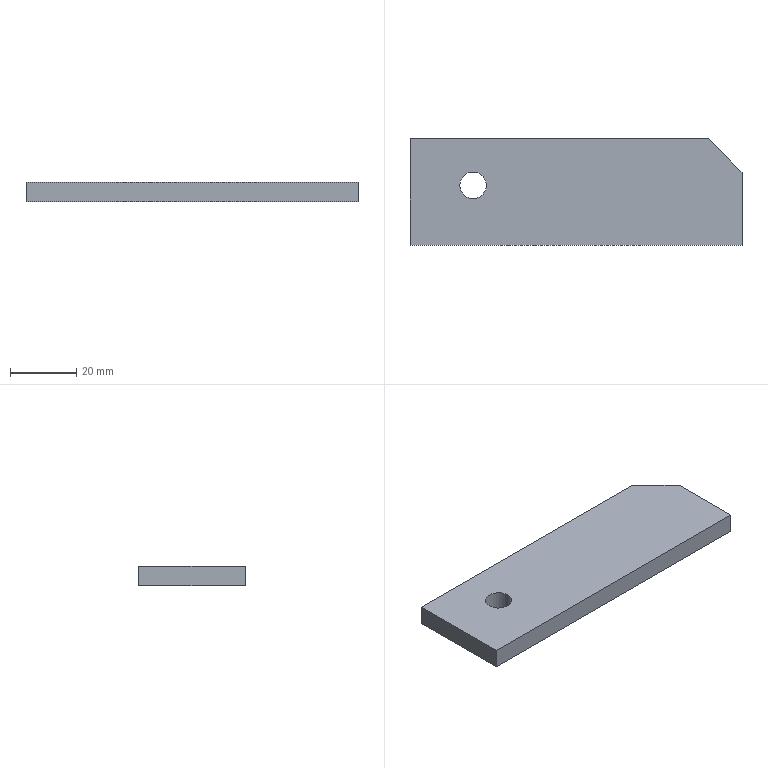Part | STEP file | [03] | 1 solid | 9 faces | box 100 x 32 x 6 mm | volume 18598 mm3 | plane 7 | cylinder 2 | commonest cylinder face diameters 8 x2
STEP:
#1=CARTESIAN_POINT('',(23.,18.,6.));
#2=VERTEX_POINT('',#1);
#3=CARTESIAN_POINT('',(15.,18.,6.));
#4=VERTEX_POINT('',#3);
#5=CARTESIAN_POINT('',(19.,18.,6.));
#6=DIRECTION('',(0.,0.,-1.));
#7=DIRECTION('',(-1.,0.,0.));
#8=AXIS2_PLACEMENT_3D('',#5,#6,#7);
#9=CIRCLE('',#8,4.);
#10=EDGE_CURVE('',#2,#4,#9,.T.);
#11=ORIENTED_EDGE('',*,*,#10,.F.);
#12=CARTESIAN_POINT('',(23.,18.,0.));
#13=VERTEX_POINT('',#12);
#14=CARTESIAN_POINT('',(23.,18.,6.));
#15=DIRECTION('',(0.,0.,-1.));
#16=VECTOR('',#15,1000.);
#17=LINE('',#14,#16);
#18=EDGE_CURVE('',#2,#13,#17,.T.);
#19=ORIENTED_EDGE('',*,*,#18,.T.);
#20=CARTESIAN_POINT('',(15.,18.,0.));
#21=VERTEX_POINT('',#20);
#22=CARTESIAN_POINT('',(19.,18.,0.));
#23=DIRECTION('',(0.,0.,1.));
#24=DIRECTION('',(1.,0.,0.));
#25=AXIS2_PLACEMENT_3D('',#22,#23,#24);
#26=CIRCLE('',#25,4.);
#27=EDGE_CURVE('',#21,#13,#26,.T.);
#28=ORIENTED_EDGE('',*,*,#27,.F.);
#29=CARTESIAN_POINT('',(15.,18.,6.));
#30=DIRECTION('',(0.,0.,-1.));
#31=VECTOR('',#30,1000.);
#32=LINE('',#29,#31);
#33=EDGE_CURVE('',#4,#21,#32,.T.);
#34=ORIENTED_EDGE('',*,*,#33,.F.);
#35=EDGE_LOOP('',(#11,#19,#28,#34));
#36=FACE_OUTER_BOUND('',#35,.T.);
#37=CARTESIAN_POINT('',(19.,18.,6.));
#38=DIRECTION('',(0.,0.,-1.));
#39=DIRECTION('',(-1.,0.,0.));
#40=AXIS2_PLACEMENT_3D('',#37,#38,#39);
#41=CYLINDRICAL_SURFACE('',#40,4.);
#42=ADVANCED_FACE('',(#36),#41,.F.);
#43=CARTESIAN_POINT('',(19.,18.,6.));
#44=DIRECTION('',(0.,0.,-1.));
#45=DIRECTION('',(-1.,0.,0.));
#46=AXIS2_PLACEMENT_3D('',#43,#44,#45);
#47=CIRCLE('',#46,4.);
#48=EDGE_CURVE('',#4,#2,#47,.T.);
#49=ORIENTED_EDGE('',*,*,#48,.T.);
#50=ORIENTED_EDGE('',*,*,#10,.T.);
#51=EDGE_LOOP('',(#49,#50));
#52=FACE_BOUND('',#51,.T.);
#53=CARTESIAN_POINT('',(100.,22.,6.));
#54=VERTEX_POINT('',#53);
#55=CARTESIAN_POINT('',(100.,0.,6.));
#56=VERTEX_POINT('',#55);
#57=CARTESIAN_POINT('',(100.,16.,6.));
#58=DIRECTION('',(0.,-1.,0.));
#59=VECTOR('',#58,1000.);
#60=LINE('',#57,#59);
#61=EDGE_CURVE('',#54,#56,#60,.T.);
#62=ORIENTED_EDGE('',*,*,#61,.F.);
#63=CARTESIAN_POINT('',(90.,32.,6.));
#64=VERTEX_POINT('',#63);
#65=CARTESIAN_POINT('',(78.,44.,6.));
#66=DIRECTION('',(-0.7071,0.7071,0.));
#67=VECTOR('',#66,1000.);
#68=LINE('',#65,#67);
#69=EDGE_CURVE('',#54,#64,#68,.T.);
#70=ORIENTED_EDGE('',*,*,#69,.T.);
#71=CARTESIAN_POINT('',(0.,32.,6.));
#72=VERTEX_POINT('',#71);
#73=CARTESIAN_POINT('',(50.,32.,6.));
#74=DIRECTION('',(1.,0.,0.));
#75=VECTOR('',#74,1000.);
#76=LINE('',#73,#75);
#77=EDGE_CURVE('',#72,#64,#76,.T.);
#78=ORIENTED_EDGE('',*,*,#77,.F.);
#79=CARTESIAN_POINT('',(0.,0.,6.));
#80=VERTEX_POINT('',#79);
#81=CARTESIAN_POINT('',(0.,16.,6.));
#82=DIRECTION('',(0.,1.,0.));
#83=VECTOR('',#82,1000.);
#84=LINE('',#81,#83);
#85=EDGE_CURVE('',#80,#72,#84,.T.);
#86=ORIENTED_EDGE('',*,*,#85,.F.);
#87=CARTESIAN_POINT('',(50.,0.,6.));
#88=DIRECTION('',(-1.,0.,0.));
#89=VECTOR('',#88,1000.);
#90=LINE('',#87,#89);
#91=EDGE_CURVE('',#56,#80,#90,.T.);
#92=ORIENTED_EDGE('',*,*,#91,.F.);
#93=EDGE_LOOP('',(#62,#70,#78,#86,#92));
#94=FACE_OUTER_BOUND('',#93,.T.);
#95=CARTESIAN_POINT('',(50.,16.,6.));
#96=DIRECTION('',(0.,0.,1.));
#97=DIRECTION('',(1.,0.,0.));
#98=AXIS2_PLACEMENT_3D('',#95,#96,#97);
#99=PLANE('',#98);
#100=ADVANCED_FACE('',(#52,#94),#99,.T.);
#101=CARTESIAN_POINT('',(100.,0.,0.));
#102=VERTEX_POINT('',#101);
#103=CARTESIAN_POINT('',(100.,0.,0.));
#104=DIRECTION('',(0.,0.,1.));
#105=VECTOR('',#104,1000.);
#106=LINE('',#103,#105);
#107=EDGE_CURVE('',#102,#56,#106,.T.);
#108=ORIENTED_EDGE('',*,*,#107,.T.);
#109=ORIENTED_EDGE('',*,*,#91,.T.);
#110=CARTESIAN_POINT('',(0.,0.,0.));
#111=VERTEX_POINT('',#110);
#112=CARTESIAN_POINT('',(0.,0.,0.));
#113=DIRECTION('',(0.,0.,1.));
#114=VECTOR('',#113,1000.);
#115=LINE('',#112,#114);
#116=EDGE_CURVE('',#111,#80,#115,.T.);
#117=ORIENTED_EDGE('',*,*,#116,.F.);
#118=CARTESIAN_POINT('',(50.,0.,0.));
#119=DIRECTION('',(1.,0.,0.));
#120=VECTOR('',#119,1000.);
#121=LINE('',#118,#120);
#122=EDGE_CURVE('',#111,#102,#121,.T.);
#123=ORIENTED_EDGE('',*,*,#122,.T.);
#124=EDGE_LOOP('',(#108,#109,#117,#123));
#125=FACE_OUTER_BOUND('',#124,.T.);
#126=CARTESIAN_POINT('',(50.,0.,0.));
#127=DIRECTION('',(0.,-1.,0.));
#128=DIRECTION('',(0.,0.,-1.));
#129=AXIS2_PLACEMENT_3D('',#126,#127,#128);
#130=PLANE('',#129);
#131=ADVANCED_FACE('',(#125),#130,.T.);
#132=ORIENTED_EDGE('',*,*,#116,.T.);
#133=ORIENTED_EDGE('',*,*,#85,.T.);
#134=CARTESIAN_POINT('',(0.,32.,0.));
#135=VERTEX_POINT('',#134);
#136=CARTESIAN_POINT('',(0.,32.,0.));
#137=DIRECTION('',(0.,0.,1.));
#138=VECTOR('',#137,1000.);
#139=LINE('',#136,#138);
#140=EDGE_CURVE('',#135,#72,#139,.T.);
#141=ORIENTED_EDGE('',*,*,#140,.F.);
#142=CARTESIAN_POINT('',(0.,16.,0.));
#143=DIRECTION('',(0.,-1.,0.));
#144=VECTOR('',#143,1000.);
#145=LINE('',#142,#144);
#146=EDGE_CURVE('',#135,#111,#145,.T.);
#147=ORIENTED_EDGE('',*,*,#146,.T.);
#148=EDGE_LOOP('',(#132,#133,#141,#147));
#149=FACE_OUTER_BOUND('',#148,.T.);
#150=CARTESIAN_POINT('',(0.,16.,0.));
#151=DIRECTION('',(-1.,0.,0.));
#152=DIRECTION('',(0.,0.,1.));
#153=AXIS2_PLACEMENT_3D('',#150,#151,#152);
#154=PLANE('',#153);
#155=ADVANCED_FACE('',(#149),#154,.T.);
#156=ORIENTED_EDGE('',*,*,#77,.T.);
#157=CARTESIAN_POINT('',(90.,32.,0.));
#158=VERTEX_POINT('',#157);
#159=CARTESIAN_POINT('',(90.,32.,0.));
#160=DIRECTION('',(0.,0.,-1.));
#161=VECTOR('',#160,1000.);
#162=LINE('',#159,#161);
#163=EDGE_CURVE('',#64,#158,#162,.T.);
#164=ORIENTED_EDGE('',*,*,#163,.T.);
#165=CARTESIAN_POINT('',(50.,32.,0.));
#166=DIRECTION('',(-1.,0.,0.));
#167=VECTOR('',#166,1000.);
#168=LINE('',#165,#167);
#169=EDGE_CURVE('',#158,#135,#168,.T.);
#170=ORIENTED_EDGE('',*,*,#169,.T.);
#171=ORIENTED_EDGE('',*,*,#140,.T.);
#172=EDGE_LOOP('',(#156,#164,#170,#171));
#173=FACE_OUTER_BOUND('',#172,.T.);
#174=CARTESIAN_POINT('',(50.,32.,0.));
#175=DIRECTION('',(0.,1.,0.));
#176=DIRECTION('',(0.,0.,1.));
#177=AXIS2_PLACEMENT_3D('',#174,#175,#176);
#178=PLANE('',#177);
#179=ADVANCED_FACE('',(#173),#178,.T.);
#180=ORIENTED_EDGE('',*,*,#27,.T.);
#181=CARTESIAN_POINT('',(19.,18.,0.));
#182=DIRECTION('',(0.,0.,1.));
#183=DIRECTION('',(1.,0.,0.));
#184=AXIS2_PLACEMENT_3D('',#181,#182,#183);
#185=CIRCLE('',#184,4.);
#186=EDGE_CURVE('',#13,#21,#185,.T.);
#187=ORIENTED_EDGE('',*,*,#186,.T.);
#188=EDGE_LOOP('',(#180,#187));
#189=FACE_BOUND('',#188,.T.);
#190=ORIENTED_EDGE('',*,*,#169,.F.);
#191=CARTESIAN_POINT('',(100.,22.,0.));
#192=VERTEX_POINT('',#191);
#193=CARTESIAN_POINT('',(78.,44.,0.));
#194=DIRECTION('',(0.7071,-0.7071,0.));
#195=VECTOR('',#194,1000.);
#196=LINE('',#193,#195);
#197=EDGE_CURVE('',#158,#192,#196,.T.);
#198=ORIENTED_EDGE('',*,*,#197,.T.);
#199=CARTESIAN_POINT('',(100.,16.,0.));
#200=DIRECTION('',(0.,1.,0.));
#201=VECTOR('',#200,1000.);
#202=LINE('',#199,#201);
#203=EDGE_CURVE('',#102,#192,#202,.T.);
#204=ORIENTED_EDGE('',*,*,#203,.F.);
#205=ORIENTED_EDGE('',*,*,#122,.F.);
#206=ORIENTED_EDGE('',*,*,#146,.F.);
#207=EDGE_LOOP('',(#190,#198,#204,#205,#206));
#208=FACE_OUTER_BOUND('',#207,.T.);
#209=CARTESIAN_POINT('',(50.,16.,0.));
#210=DIRECTION('',(0.,0.,-1.));
#211=DIRECTION('',(-1.,0.,0.));
#212=AXIS2_PLACEMENT_3D('',#209,#210,#211);
#213=PLANE('',#212);
#214=ADVANCED_FACE('',(#189,#208),#213,.T.);
#215=ORIENTED_EDGE('',*,*,#203,.T.);
#216=CARTESIAN_POINT('',(100.,22.,0.));
#217=DIRECTION('',(0.,0.,1.));
#218=VECTOR('',#217,1000.);
#219=LINE('',#216,#218);
#220=EDGE_CURVE('',#192,#54,#219,.T.);
#221=ORIENTED_EDGE('',*,*,#220,.T.);
#222=ORIENTED_EDGE('',*,*,#61,.T.);
#223=ORIENTED_EDGE('',*,*,#107,.F.);
#224=EDGE_LOOP('',(#215,#221,#222,#223));
#225=FACE_OUTER_BOUND('',#224,.T.);
#226=CARTESIAN_POINT('',(100.,16.,0.));
#227=DIRECTION('',(1.,0.,0.));
#228=DIRECTION('',(0.,0.,-1.));
#229=AXIS2_PLACEMENT_3D('',#226,#227,#228);
#230=PLANE('',#229);
#231=ADVANCED_FACE('',(#225),#230,.T.);
#232=ORIENTED_EDGE('',*,*,#197,.F.);
#233=ORIENTED_EDGE('',*,*,#163,.F.);
#234=ORIENTED_EDGE('',*,*,#69,.F.);
#235=ORIENTED_EDGE('',*,*,#220,.F.);
#236=EDGE_LOOP('',(#232,#233,#234,#235));
#237=FACE_OUTER_BOUND('',#236,.T.);
#238=CARTESIAN_POINT('',(100.,22.,0.));
#239=DIRECTION('',(-0.7071,-0.7071,0.));
#240=DIRECTION('',(0.,0.,1.));
#241=AXIS2_PLACEMENT_3D('',#238,#239,#240);
#242=PLANE('',#241);
#243=ADVANCED_FACE('',(#237),#242,.F.);
#244=ORIENTED_EDGE('',*,*,#18,.F.);
#245=ORIENTED_EDGE('',*,*,#48,.F.);
#246=ORIENTED_EDGE('',*,*,#33,.T.);
#247=ORIENTED_EDGE('',*,*,#186,.F.);
#248=EDGE_LOOP('',(#244,#245,#246,#247));
#249=FACE_OUTER_BOUND('',#248,.T.);
#250=CARTESIAN_POINT('',(19.,18.,6.));
#251=DIRECTION('',(0.,0.,-1.));
#252=DIRECTION('',(-1.,0.,0.));
#253=AXIS2_PLACEMENT_3D('',#250,#251,#252);
#254=CYLINDRICAL_SURFACE('',#253,4.);
#255=ADVANCED_FACE('',(#249),#254,.F.);
#256=CLOSED_SHELL('',(#42,#100,#131,#155,#179,#214,#231,#243,#255));
#257=MANIFOLD_SOLID_BREP('',#256);
#258=CARTESIAN_POINT('',(0.,0.,0.));
#259=DIRECTION('',(0.,0.,1.));
#260=DIRECTION('',(1.,0.,0.));
#261=AXIS2_PLACEMENT_3D('',#258,#259,#260);
#262=(LENGTH_UNIT()NAMED_UNIT(*)SI_UNIT(.MILLI.,.METRE.));
#263=UNCERTAINTY_MEASURE_WITH_UNIT(LENGTH_MEASURE(0.00001),#262,'','');
#264=(NAMED_UNIT(*)PLANE_ANGLE_UNIT()SI_UNIT($,.RADIAN.));
#265=(NAMED_UNIT(*)SI_UNIT($,.STERADIAN.)SOLID_ANGLE_UNIT());
#266=(GEOMETRIC_REPRESENTATION_CONTEXT(3)GLOBAL_UNCERTAINTY_ASSIGNED_CONTEXT((#263))GLOBAL_UNIT_ASSIGNED_CONTEXT((#262,#264,#265))REPRESENTATION_CONTEXT('',''));
#267=ADVANCED_BREP_SHAPE_REPRESENTATION('',(#257,#261),#266);